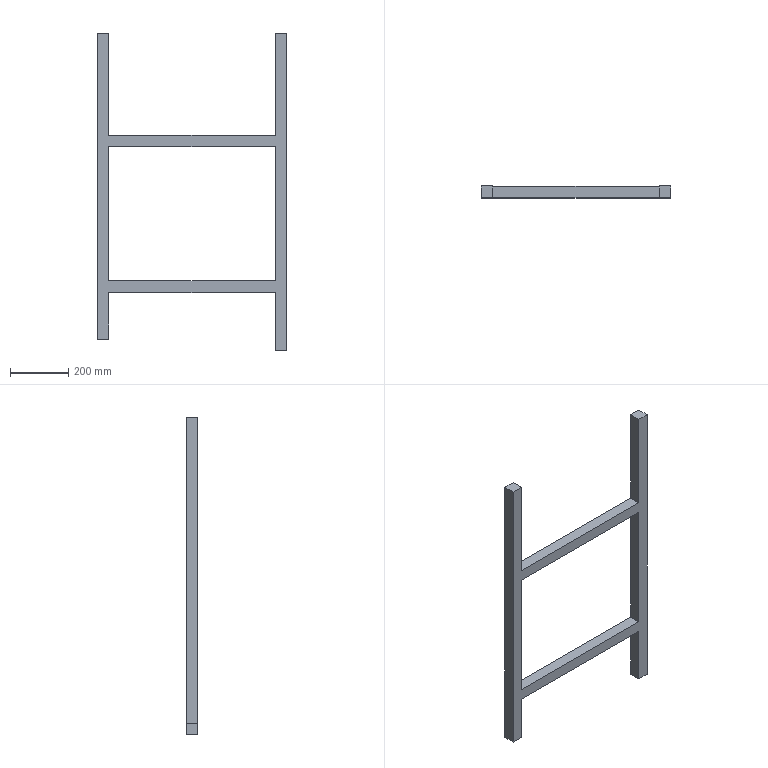Part | NX | features 凸台-拉伸23 2 | 1 solid | 18 faces | box 650 x 40 x 1090 mm | volume 5248000 mm3 | plane 18
STEP:
#1=CARTESIAN_POINT('',(3933.,-40.,-902.985));
#2=VERTEX_POINT('',#1);
#3=CARTESIAN_POINT('',(3933.,0.,-902.985));
#4=VERTEX_POINT('',#3);
#5=CARTESIAN_POINT('',(3933.,0.,-902.985));
#6=DIRECTION('',(0.,1.,0.));
#7=VECTOR('',#6,1000.);
#8=LINE('',#5,#7);
#9=EDGE_CURVE('',#2,#4,#8,.T.);
#10=ORIENTED_EDGE('',*,*,#9,.F.);
#11=CARTESIAN_POINT('',(3363.,-40.,-902.985));
#12=VERTEX_POINT('',#11);
#13=CARTESIAN_POINT('',(3989.569,-40.,-902.985));
#14=DIRECTION('',(-1.,0.,0.));
#15=VECTOR('',#14,1000.);
#16=LINE('',#13,#15);
#17=EDGE_CURVE('',#2,#12,#16,.T.);
#18=ORIENTED_EDGE('',*,*,#17,.T.);
#19=CARTESIAN_POINT('',(3363.,0.,-902.985));
#20=VERTEX_POINT('',#19);
#21=CARTESIAN_POINT('',(3363.,0.,-902.985));
#22=DIRECTION('',(0.,1.,0.));
#23=VECTOR('',#22,1000.);
#24=LINE('',#21,#23);
#25=EDGE_CURVE('',#12,#20,#24,.T.);
#26=ORIENTED_EDGE('',*,*,#25,.T.);
#27=CARTESIAN_POINT('',(3989.569,0.,-902.985));
#28=DIRECTION('',(-1.,0.,0.));
#29=VECTOR('',#28,1000.);
#30=LINE('',#27,#29);
#31=EDGE_CURVE('',#4,#20,#30,.T.);
#32=ORIENTED_EDGE('',*,*,#31,.F.);
#33=EDGE_LOOP('',(#10,#18,#26,#32));
#34=FACE_BOUND('',#33,.T.);
#35=CARTESIAN_POINT('',(3989.569,0.,-902.985));
#36=DIRECTION('',(0.,0.,1.));
#37=DIRECTION('',(1.,0.,0.));
#38=AXIS2_PLACEMENT_3D('',#35,#36,#37);
#39=PLANE('',#38);
#40=ADVANCED_FACE('',(#34),#39,.F.);
#41=CARTESIAN_POINT('',(3933.,0.,-862.985));
#42=VERTEX_POINT('',#41);
#43=CARTESIAN_POINT('',(3933.,-40.,-862.985));
#44=VERTEX_POINT('',#43);
#45=CARTESIAN_POINT('',(3933.,0.,-862.985));
#46=DIRECTION('',(0.,-1.,0.));
#47=VECTOR('',#46,1000.);
#48=LINE('',#45,#47);
#49=EDGE_CURVE('',#42,#44,#48,.T.);
#50=ORIENTED_EDGE('',*,*,#49,.F.);
#51=CARTESIAN_POINT('',(3363.,0.,-862.985));
#52=VERTEX_POINT('',#51);
#53=CARTESIAN_POINT('',(3989.569,0.,-862.985));
#54=DIRECTION('',(-1.,0.,0.));
#55=VECTOR('',#54,1000.);
#56=LINE('',#53,#55);
#57=EDGE_CURVE('',#42,#52,#56,.T.);
#58=ORIENTED_EDGE('',*,*,#57,.T.);
#59=CARTESIAN_POINT('',(3363.,-40.,-862.985));
#60=VERTEX_POINT('',#59);
#61=CARTESIAN_POINT('',(3363.,0.,-862.985));
#62=DIRECTION('',(0.,-1.,0.));
#63=VECTOR('',#62,1000.);
#64=LINE('',#61,#63);
#65=EDGE_CURVE('',#52,#60,#64,.T.);
#66=ORIENTED_EDGE('',*,*,#65,.T.);
#67=CARTESIAN_POINT('',(3989.569,-40.,-862.985));
#68=DIRECTION('',(-1.,0.,0.));
#69=VECTOR('',#68,1000.);
#70=LINE('',#67,#69);
#71=EDGE_CURVE('',#44,#60,#70,.T.);
#72=ORIENTED_EDGE('',*,*,#71,.F.);
#73=EDGE_LOOP('',(#50,#58,#66,#72));
#74=FACE_BOUND('',#73,.T.);
#75=CARTESIAN_POINT('',(3989.569,0.,-862.985));
#76=DIRECTION('',(0.,0.,-1.));
#77=DIRECTION('',(-1.,0.,0.));
#78=AXIS2_PLACEMENT_3D('',#75,#76,#77);
#79=PLANE('',#78);
#80=ADVANCED_FACE('',(#74),#79,.F.);
#81=CARTESIAN_POINT('',(3363.,0.,-12.985));
#82=VERTEX_POINT('',#81);
#83=CARTESIAN_POINT('',(3323.,0.,-12.985));
#84=VERTEX_POINT('',#83);
#85=CARTESIAN_POINT('',(3323.,0.,-12.985));
#86=DIRECTION('',(-1.,0.,0.));
#87=VECTOR('',#86,1000.);
#88=LINE('',#85,#87);
#89=EDGE_CURVE('',#82,#84,#88,.T.);
#90=ORIENTED_EDGE('',*,*,#89,.T.);
#91=CARTESIAN_POINT('',(3323.,-40.,-12.985));
#92=VERTEX_POINT('',#91);
#93=CARTESIAN_POINT('',(3323.,0.,-12.985));
#94=DIRECTION('',(0.,-1.,0.));
#95=VECTOR('',#94,1000.);
#96=LINE('',#93,#95);
#97=EDGE_CURVE('',#84,#92,#96,.T.);
#98=ORIENTED_EDGE('',*,*,#97,.T.);
#99=CARTESIAN_POINT('',(3363.,-40.,-12.985));
#100=VERTEX_POINT('',#99);
#101=CARTESIAN_POINT('',(3323.,-40.,-12.985));
#102=DIRECTION('',(1.,0.,0.));
#103=VECTOR('',#102,1000.);
#104=LINE('',#101,#103);
#105=EDGE_CURVE('',#92,#100,#104,.T.);
#106=ORIENTED_EDGE('',*,*,#105,.T.);
#107=CARTESIAN_POINT('',(3363.,0.,-12.985));
#108=DIRECTION('',(0.,1.,0.));
#109=VECTOR('',#108,1000.);
#110=LINE('',#107,#109);
#111=EDGE_CURVE('',#100,#82,#110,.T.);
#112=ORIENTED_EDGE('',*,*,#111,.T.);
#113=EDGE_LOOP('',(#90,#98,#106,#112));
#114=FACE_BOUND('',#113,.T.);
#115=CARTESIAN_POINT('',(4349.569,0.,-12.985));
#116=DIRECTION('',(0.,0.,1.));
#117=DIRECTION('',(1.,0.,0.));
#118=AXIS2_PLACEMENT_3D('',#115,#116,#117);
#119=PLANE('',#118);
#120=ADVANCED_FACE('',(#114),#119,.T.);
#121=CARTESIAN_POINT('',(3323.,0.,-1062.985));
#122=VERTEX_POINT('',#121);
#123=CARTESIAN_POINT('',(3323.,-40.,-1062.985));
#124=VERTEX_POINT('',#123);
#125=CARTESIAN_POINT('',(3323.,0.,-1062.985));
#126=DIRECTION('',(0.,-1.,0.));
#127=VECTOR('',#126,1000.);
#128=LINE('',#125,#127);
#129=EDGE_CURVE('',#122,#124,#128,.T.);
#130=ORIENTED_EDGE('',*,*,#129,.F.);
#131=CARTESIAN_POINT('',(3363.,0.,-1062.985));
#132=VERTEX_POINT('',#131);
#133=CARTESIAN_POINT('',(3323.,0.,-1062.985));
#134=DIRECTION('',(-1.,0.,0.));
#135=VECTOR('',#134,1000.);
#136=LINE('',#133,#135);
#137=EDGE_CURVE('',#132,#122,#136,.T.);
#138=ORIENTED_EDGE('',*,*,#137,.F.);
#139=CARTESIAN_POINT('',(3363.,-40.,-1062.985));
#140=VERTEX_POINT('',#139);
#141=CARTESIAN_POINT('',(3363.,0.,-1062.985));
#142=DIRECTION('',(0.,1.,0.));
#143=VECTOR('',#142,1000.);
#144=LINE('',#141,#143);
#145=EDGE_CURVE('',#140,#132,#144,.T.);
#146=ORIENTED_EDGE('',*,*,#145,.F.);
#147=CARTESIAN_POINT('',(3323.,-40.,-1062.985));
#148=DIRECTION('',(1.,0.,0.));
#149=VECTOR('',#148,1000.);
#150=LINE('',#147,#149);
#151=EDGE_CURVE('',#124,#140,#150,.T.);
#152=ORIENTED_EDGE('',*,*,#151,.F.);
#153=EDGE_LOOP('',(#130,#138,#146,#152));
#154=FACE_BOUND('',#153,.T.);
#155=CARTESIAN_POINT('',(3000.,0.,-1062.985));
#156=DIRECTION('',(0.,0.,1.));
#157=DIRECTION('',(1.,0.,0.));
#158=AXIS2_PLACEMENT_3D('',#155,#156,#157);
#159=PLANE('',#158);
#160=ADVANCED_FACE('',(#154),#159,.F.);
#161=ORIENTED_EDGE('',*,*,#97,.F.);
#162=CARTESIAN_POINT('',(3323.,0.,43.584));
#163=DIRECTION('',(0.,0.,-1.));
#164=VECTOR('',#163,1000.);
#165=LINE('',#162,#164);
#166=EDGE_CURVE('',#84,#122,#165,.T.);
#167=ORIENTED_EDGE('',*,*,#166,.T.);
#168=ORIENTED_EDGE('',*,*,#129,.T.);
#169=CARTESIAN_POINT('',(3323.,-40.,43.584));
#170=DIRECTION('',(0.,0.,-1.));
#171=VECTOR('',#170,1000.);
#172=LINE('',#169,#171);
#173=EDGE_CURVE('',#92,#124,#172,.T.);
#174=ORIENTED_EDGE('',*,*,#173,.F.);
#175=EDGE_LOOP('',(#161,#167,#168,#174));
#176=FACE_BOUND('',#175,.T.);
#177=CARTESIAN_POINT('',(3323.,0.,43.584));
#178=DIRECTION('',(1.,0.,0.));
#179=DIRECTION('',(0.,1.,0.));
#180=AXIS2_PLACEMENT_3D('',#177,#178,#179);
#181=PLANE('',#180);
#182=ADVANCED_FACE('',(#176),#181,.F.);
#183=CARTESIAN_POINT('',(3363.,0.,-362.985));
#184=VERTEX_POINT('',#183);
#185=CARTESIAN_POINT('',(3363.,-40.,-362.985));
#186=VERTEX_POINT('',#185);
#187=CARTESIAN_POINT('',(3363.,0.,-362.985));
#188=DIRECTION('',(0.,-1.,0.));
#189=VECTOR('',#188,1000.);
#190=LINE('',#187,#189);
#191=EDGE_CURVE('',#184,#186,#190,.T.);
#192=ORIENTED_EDGE('',*,*,#191,.F.);
#193=CARTESIAN_POINT('',(3363.,0.,43.584));
#194=DIRECTION('',(0.,0.,-1.));
#195=VECTOR('',#194,1000.);
#196=LINE('',#193,#195);
#197=EDGE_CURVE('',#82,#184,#196,.T.);
#198=ORIENTED_EDGE('',*,*,#197,.F.);
#199=ORIENTED_EDGE('',*,*,#111,.F.);
#200=CARTESIAN_POINT('',(3363.,-40.,43.584));
#201=DIRECTION('',(0.,0.,-1.));
#202=VECTOR('',#201,1000.);
#203=LINE('',#200,#202);
#204=EDGE_CURVE('',#100,#186,#203,.T.);
#205=ORIENTED_EDGE('',*,*,#204,.T.);
#206=EDGE_LOOP('',(#192,#198,#199,#205));
#207=FACE_BOUND('',#206,.T.);
#208=CARTESIAN_POINT('',(3363.,0.,43.584));
#209=DIRECTION('',(-1.,0.,0.));
#210=DIRECTION('',(0.,-1.,0.));
#211=AXIS2_PLACEMENT_3D('',#208,#209,#210);
#212=PLANE('',#211);
#213=ADVANCED_FACE('',(#207),#212,.F.);
#214=CARTESIAN_POINT('',(3933.,-40.,-402.985));
#215=VERTEX_POINT('',#214);
#216=CARTESIAN_POINT('',(3933.,0.,-402.985));
#217=VERTEX_POINT('',#216);
#218=CARTESIAN_POINT('',(3933.,0.,-402.985));
#219=DIRECTION('',(0.,1.,0.));
#220=VECTOR('',#219,1000.);
#221=LINE('',#218,#220);
#222=EDGE_CURVE('',#215,#217,#221,.T.);
#223=ORIENTED_EDGE('',*,*,#222,.F.);
#224=CARTESIAN_POINT('',(3363.,-40.,-402.985));
#225=VERTEX_POINT('',#224);
#226=CARTESIAN_POINT('',(3989.569,-40.,-402.985));
#227=DIRECTION('',(-1.,0.,0.));
#228=VECTOR('',#227,1000.);
#229=LINE('',#226,#228);
#230=EDGE_CURVE('',#215,#225,#229,.T.);
#231=ORIENTED_EDGE('',*,*,#230,.T.);
#232=CARTESIAN_POINT('',(3363.,0.,-402.985));
#233=VERTEX_POINT('',#232);
#234=CARTESIAN_POINT('',(3363.,0.,-402.985));
#235=DIRECTION('',(0.,1.,0.));
#236=VECTOR('',#235,1000.);
#237=LINE('',#234,#236);
#238=EDGE_CURVE('',#225,#233,#237,.T.);
#239=ORIENTED_EDGE('',*,*,#238,.T.);
#240=CARTESIAN_POINT('',(3989.569,0.,-402.985));
#241=DIRECTION('',(-1.,0.,0.));
#242=VECTOR('',#241,1000.);
#243=LINE('',#240,#242);
#244=EDGE_CURVE('',#217,#233,#243,.T.);
#245=ORIENTED_EDGE('',*,*,#244,.F.);
#246=EDGE_LOOP('',(#223,#231,#239,#245));
#247=FACE_BOUND('',#246,.T.);
#248=CARTESIAN_POINT('',(3989.569,0.,-402.985));
#249=DIRECTION('',(0.,0.,1.));
#250=DIRECTION('',(1.,0.,0.));
#251=AXIS2_PLACEMENT_3D('',#248,#249,#250);
#252=PLANE('',#251);
#253=ADVANCED_FACE('',(#247),#252,.F.);
#254=CARTESIAN_POINT('',(3933.,0.,-362.985));
#255=VERTEX_POINT('',#254);
#256=CARTESIAN_POINT('',(3933.,-40.,-362.985));
#257=VERTEX_POINT('',#256);
#258=CARTESIAN_POINT('',(3933.,0.,-362.985));
#259=DIRECTION('',(0.,-1.,0.));
#260=VECTOR('',#259,1000.);
#261=LINE('',#258,#260);
#262=EDGE_CURVE('',#255,#257,#261,.T.);
#263=ORIENTED_EDGE('',*,*,#262,.F.);
#264=CARTESIAN_POINT('',(3989.569,0.,-362.985));
#265=DIRECTION('',(-1.,0.,0.));
#266=VECTOR('',#265,1000.);
#267=LINE('',#264,#266);
#268=EDGE_CURVE('',#255,#184,#267,.T.);
#269=ORIENTED_EDGE('',*,*,#268,.T.);
#270=ORIENTED_EDGE('',*,*,#191,.T.);
#271=CARTESIAN_POINT('',(3989.569,-40.,-362.985));
#272=DIRECTION('',(-1.,0.,0.));
#273=VECTOR('',#272,1000.);
#274=LINE('',#271,#273);
#275=EDGE_CURVE('',#257,#186,#274,.T.);
#276=ORIENTED_EDGE('',*,*,#275,.F.);
#277=EDGE_LOOP('',(#263,#269,#270,#276));
#278=FACE_BOUND('',#277,.T.);
#279=CARTESIAN_POINT('',(3989.569,0.,-362.985));
#280=DIRECTION('',(0.,0.,-1.));
#281=DIRECTION('',(-1.,0.,0.));
#282=AXIS2_PLACEMENT_3D('',#279,#280,#281);
#283=PLANE('',#282);
#284=ADVANCED_FACE('',(#278),#283,.F.);
#285=CARTESIAN_POINT('',(3973.,0.,-1102.985));
#286=VERTEX_POINT('',#285);
#287=CARTESIAN_POINT('',(3933.,0.,-1102.985));
#288=VERTEX_POINT('',#287);
#289=CARTESIAN_POINT('',(3933.,0.,-1102.985));
#290=DIRECTION('',(-1.,0.,0.));
#291=VECTOR('',#290,1000.);
#292=LINE('',#289,#291);
#293=EDGE_CURVE('',#286,#288,#292,.T.);
#294=ORIENTED_EDGE('',*,*,#293,.F.);
#295=CARTESIAN_POINT('',(3973.,-40.,-1102.985));
#296=VERTEX_POINT('',#295);
#297=CARTESIAN_POINT('',(3973.,-40.,-1102.985));
#298=DIRECTION('',(0.,1.,0.));
#299=VECTOR('',#298,1000.);
#300=LINE('',#297,#299);
#301=EDGE_CURVE('',#296,#286,#300,.T.);
#302=ORIENTED_EDGE('',*,*,#301,.F.);
#303=CARTESIAN_POINT('',(3933.,-40.,-1102.985));
#304=VERTEX_POINT('',#303);
#305=CARTESIAN_POINT('',(3933.,-40.,-1102.985));
#306=DIRECTION('',(1.,0.,0.));
#307=VECTOR('',#306,1000.);
#308=LINE('',#305,#307);
#309=EDGE_CURVE('',#304,#296,#308,.T.);
#310=ORIENTED_EDGE('',*,*,#309,.F.);
#311=CARTESIAN_POINT('',(3933.,-40.,-1102.985));
#312=DIRECTION('',(0.,-1.,0.));
#313=VECTOR('',#312,1000.);
#314=LINE('',#311,#313);
#315=EDGE_CURVE('',#288,#304,#314,.T.);
#316=ORIENTED_EDGE('',*,*,#315,.F.);
#317=EDGE_LOOP('',(#294,#302,#310,#316));
#318=FACE_BOUND('',#317,.T.);
#319=CARTESIAN_POINT('',(4349.569,-560.,-1102.985));
#320=DIRECTION('',(0.,0.,1.));
#321=DIRECTION('',(1.,0.,0.));
#322=AXIS2_PLACEMENT_3D('',#319,#320,#321);
#323=PLANE('',#322);
#324=ADVANCED_FACE('',(#318),#323,.F.);
#325=CARTESIAN_POINT('',(3973.,0.,-12.985));
#326=VERTEX_POINT('',#325);
#327=CARTESIAN_POINT('',(3973.,0.,-1159.553));
#328=DIRECTION('',(0.,0.,1.));
#329=VECTOR('',#328,1000.);
#330=LINE('',#327,#329);
#331=EDGE_CURVE('',#286,#326,#330,.T.);
#332=ORIENTED_EDGE('',*,*,#331,.F.);
#333=ORIENTED_EDGE('',*,*,#293,.T.);
#334=CARTESIAN_POINT('',(3933.,0.,-1159.553));
#335=DIRECTION('',(0.,0.,1.));
#336=VECTOR('',#335,1000.);
#337=LINE('',#334,#336);
#338=EDGE_CURVE('',#288,#4,#337,.T.);
#339=ORIENTED_EDGE('',*,*,#338,.T.);
#340=ORIENTED_EDGE('',*,*,#31,.T.);
#341=CARTESIAN_POINT('',(3363.,0.,43.584));
#342=DIRECTION('',(0.,0.,-1.));
#343=VECTOR('',#342,1000.);
#344=LINE('',#341,#343);
#345=EDGE_CURVE('',#20,#132,#344,.T.);
#346=ORIENTED_EDGE('',*,*,#345,.T.);
#347=ORIENTED_EDGE('',*,*,#137,.T.);
#348=ORIENTED_EDGE('',*,*,#166,.F.);
#349=ORIENTED_EDGE('',*,*,#89,.F.);
#350=ORIENTED_EDGE('',*,*,#197,.T.);
#351=ORIENTED_EDGE('',*,*,#268,.F.);
#352=CARTESIAN_POINT('',(3933.,0.,-12.985));
#353=VERTEX_POINT('',#352);
#354=CARTESIAN_POINT('',(3933.,0.,-1159.553));
#355=DIRECTION('',(0.,0.,1.));
#356=VECTOR('',#355,1000.);
#357=LINE('',#354,#356);
#358=EDGE_CURVE('',#255,#353,#357,.T.);
#359=ORIENTED_EDGE('',*,*,#358,.T.);
#360=CARTESIAN_POINT('',(3933.,0.,-12.985));
#361=DIRECTION('',(1.,0.,0.));
#362=VECTOR('',#361,1000.);
#363=LINE('',#360,#362);
#364=EDGE_CURVE('',#353,#326,#363,.T.);
#365=ORIENTED_EDGE('',*,*,#364,.T.);
#366=EDGE_LOOP('',(#332,#333,#339,#340,#346,#347,#348,#349,#350,#351,#359,#365));
#367=FACE_BOUND('',#366,.T.);
#368=ORIENTED_EDGE('',*,*,#57,.F.);
#369=CARTESIAN_POINT('',(3933.,0.,-1159.553));
#370=DIRECTION('',(0.,0.,1.));
#371=VECTOR('',#370,1000.);
#372=LINE('',#369,#371);
#373=EDGE_CURVE('',#42,#217,#372,.T.);
#374=ORIENTED_EDGE('',*,*,#373,.T.);
#375=ORIENTED_EDGE('',*,*,#244,.T.);
#376=CARTESIAN_POINT('',(3363.,0.,43.584));
#377=DIRECTION('',(0.,0.,-1.));
#378=VECTOR('',#377,1000.);
#379=LINE('',#376,#378);
#380=EDGE_CURVE('',#233,#52,#379,.T.);
#381=ORIENTED_EDGE('',*,*,#380,.T.);
#382=EDGE_LOOP('',(#368,#374,#375,#381));
#383=FACE_BOUND('',#382,.T.);
#384=CARTESIAN_POINT('',(3933.,0.,-1159.553));
#385=DIRECTION('',(0.,-1.,0.));
#386=DIRECTION('',(1.,0.,0.));
#387=AXIS2_PLACEMENT_3D('',#384,#385,#386);
#388=PLANE('',#387);
#389=ADVANCED_FACE('',(#367,#383),#388,.F.);
#390=CARTESIAN_POINT('',(3973.,-40.,-12.985));
#391=VERTEX_POINT('',#390);
#392=CARTESIAN_POINT('',(3973.,-40.,-1159.553));
#393=DIRECTION('',(0.,0.,1.));
#394=VECTOR('',#393,1000.);
#395=LINE('',#392,#394);
#396=EDGE_CURVE('',#296,#391,#395,.T.);
#397=ORIENTED_EDGE('',*,*,#396,.F.);
#398=ORIENTED_EDGE('',*,*,#301,.T.);
#399=ORIENTED_EDGE('',*,*,#331,.T.);
#400=CARTESIAN_POINT('',(3973.,-40.,-12.985));
#401=DIRECTION('',(0.,-1.,0.));
#402=VECTOR('',#401,1000.);
#403=LINE('',#400,#402);
#404=EDGE_CURVE('',#326,#391,#403,.T.);
#405=ORIENTED_EDGE('',*,*,#404,.T.);
#406=EDGE_LOOP('',(#397,#398,#399,#405));
#407=FACE_BOUND('',#406,.T.);
#408=CARTESIAN_POINT('',(3973.,-40.,-1159.553));
#409=DIRECTION('',(-1.,0.,0.));
#410=DIRECTION('',(0.,0.,1.));
#411=AXIS2_PLACEMENT_3D('',#408,#409,#410);
#412=PLANE('',#411);
#413=ADVANCED_FACE('',(#407),#412,.F.);
#414=CARTESIAN_POINT('',(3933.,-40.,-1159.553));
#415=DIRECTION('',(0.,0.,1.));
#416=VECTOR('',#415,1000.);
#417=LINE('',#414,#416);
#418=EDGE_CURVE('',#44,#215,#417,.T.);
#419=ORIENTED_EDGE('',*,*,#418,.F.);
#420=ORIENTED_EDGE('',*,*,#71,.T.);
#421=CARTESIAN_POINT('',(3363.,-40.,43.584));
#422=DIRECTION('',(0.,0.,-1.));
#423=VECTOR('',#422,1000.);
#424=LINE('',#421,#423);
#425=EDGE_CURVE('',#225,#60,#424,.T.);
#426=ORIENTED_EDGE('',*,*,#425,.F.);
#427=ORIENTED_EDGE('',*,*,#230,.F.);
#428=EDGE_LOOP('',(#419,#420,#426,#427));
#429=FACE_BOUND('',#428,.T.);
#430=ORIENTED_EDGE('',*,*,#17,.F.);
#431=CARTESIAN_POINT('',(3933.,-40.,-1159.553));
#432=DIRECTION('',(0.,0.,1.));
#433=VECTOR('',#432,1000.);
#434=LINE('',#431,#433);
#435=EDGE_CURVE('',#304,#2,#434,.T.);
#436=ORIENTED_EDGE('',*,*,#435,.F.);
#437=ORIENTED_EDGE('',*,*,#309,.T.);
#438=ORIENTED_EDGE('',*,*,#396,.T.);
#439=CARTESIAN_POINT('',(3933.,-40.,-12.985));
#440=VERTEX_POINT('',#439);
#441=CARTESIAN_POINT('',(3933.,-40.,-12.985));
#442=DIRECTION('',(-1.,0.,0.));
#443=VECTOR('',#442,1000.);
#444=LINE('',#441,#443);
#445=EDGE_CURVE('',#391,#440,#444,.T.);
#446=ORIENTED_EDGE('',*,*,#445,.T.);
#447=CARTESIAN_POINT('',(3933.,-40.,-1159.553));
#448=DIRECTION('',(0.,0.,1.));
#449=VECTOR('',#448,1000.);
#450=LINE('',#447,#449);
#451=EDGE_CURVE('',#257,#440,#450,.T.);
#452=ORIENTED_EDGE('',*,*,#451,.F.);
#453=ORIENTED_EDGE('',*,*,#275,.T.);
#454=ORIENTED_EDGE('',*,*,#204,.F.);
#455=ORIENTED_EDGE('',*,*,#105,.F.);
#456=ORIENTED_EDGE('',*,*,#173,.T.);
#457=ORIENTED_EDGE('',*,*,#151,.T.);
#458=CARTESIAN_POINT('',(3363.,-40.,43.584));
#459=DIRECTION('',(0.,0.,-1.));
#460=VECTOR('',#459,1000.);
#461=LINE('',#458,#460);
#462=EDGE_CURVE('',#12,#140,#461,.T.);
#463=ORIENTED_EDGE('',*,*,#462,.F.);
#464=EDGE_LOOP('',(#430,#436,#437,#438,#446,#452,#453,#454,#455,#456,#457,#463));
#465=FACE_BOUND('',#464,.T.);
#466=CARTESIAN_POINT('',(3933.,-40.,-1159.553));
#467=DIRECTION('',(0.,1.,0.));
#468=DIRECTION('',(-1.,0.,0.));
#469=AXIS2_PLACEMENT_3D('',#466,#467,#468);
#470=PLANE('',#469);
#471=ADVANCED_FACE('',(#429,#465),#470,.F.);
#472=CARTESIAN_POINT('',(3933.,-40.,-12.985));
#473=DIRECTION('',(0.,1.,0.));
#474=VECTOR('',#473,1000.);
#475=LINE('',#472,#474);
#476=EDGE_CURVE('',#440,#353,#475,.T.);
#477=ORIENTED_EDGE('',*,*,#476,.F.);
#478=ORIENTED_EDGE('',*,*,#445,.F.);
#479=ORIENTED_EDGE('',*,*,#404,.F.);
#480=ORIENTED_EDGE('',*,*,#364,.F.);
#481=EDGE_LOOP('',(#477,#478,#479,#480));
#482=FACE_BOUND('',#481,.T.);
#483=CARTESIAN_POINT('',(3000.,0.,-12.985));
#484=DIRECTION('',(0.,0.,-1.));
#485=DIRECTION('',(-1.,0.,0.));
#486=AXIS2_PLACEMENT_3D('',#483,#484,#485);
#487=PLANE('',#486);
#488=ADVANCED_FACE('',(#482),#487,.F.);
#489=ORIENTED_EDGE('',*,*,#358,.F.);
#490=ORIENTED_EDGE('',*,*,#262,.T.);
#491=ORIENTED_EDGE('',*,*,#451,.T.);
#492=ORIENTED_EDGE('',*,*,#476,.T.);
#493=EDGE_LOOP('',(#489,#490,#491,#492));
#494=FACE_BOUND('',#493,.T.);
#495=CARTESIAN_POINT('',(3933.,-40.,-1159.553));
#496=DIRECTION('',(1.,0.,0.));
#497=DIRECTION('',(0.,0.,-1.));
#498=AXIS2_PLACEMENT_3D('',#495,#496,#497);
#499=PLANE('',#498);
#500=ADVANCED_FACE('',(#494),#499,.F.);
#501=ORIENTED_EDGE('',*,*,#25,.F.);
#502=ORIENTED_EDGE('',*,*,#462,.T.);
#503=ORIENTED_EDGE('',*,*,#145,.T.);
#504=ORIENTED_EDGE('',*,*,#345,.F.);
#505=EDGE_LOOP('',(#501,#502,#503,#504));
#506=FACE_BOUND('',#505,.T.);
#507=CARTESIAN_POINT('',(3363.,0.,43.584));
#508=DIRECTION('',(-1.,0.,0.));
#509=DIRECTION('',(0.,-1.,0.));
#510=AXIS2_PLACEMENT_3D('',#507,#508,#509);
#511=PLANE('',#510);
#512=ADVANCED_FACE('',(#506),#511,.F.);
#513=ORIENTED_EDGE('',*,*,#65,.F.);
#514=ORIENTED_EDGE('',*,*,#380,.F.);
#515=ORIENTED_EDGE('',*,*,#238,.F.);
#516=ORIENTED_EDGE('',*,*,#425,.T.);
#517=EDGE_LOOP('',(#513,#514,#515,#516));
#518=FACE_BOUND('',#517,.T.);
#519=CARTESIAN_POINT('',(3363.,0.,43.584));
#520=DIRECTION('',(-1.,0.,0.));
#521=DIRECTION('',(0.,-1.,0.));
#522=AXIS2_PLACEMENT_3D('',#519,#520,#521);
#523=PLANE('',#522);
#524=ADVANCED_FACE('',(#518),#523,.F.);
#525=ORIENTED_EDGE('',*,*,#9,.T.);
#526=ORIENTED_EDGE('',*,*,#338,.F.);
#527=ORIENTED_EDGE('',*,*,#315,.T.);
#528=ORIENTED_EDGE('',*,*,#435,.T.);
#529=EDGE_LOOP('',(#525,#526,#527,#528));
#530=FACE_BOUND('',#529,.T.);
#531=CARTESIAN_POINT('',(3933.,-40.,-1159.553));
#532=DIRECTION('',(1.,0.,0.));
#533=DIRECTION('',(0.,0.,-1.));
#534=AXIS2_PLACEMENT_3D('',#531,#532,#533);
#535=PLANE('',#534);
#536=ADVANCED_FACE('',(#530),#535,.F.);
#537=ORIENTED_EDGE('',*,*,#49,.T.);
#538=ORIENTED_EDGE('',*,*,#418,.T.);
#539=ORIENTED_EDGE('',*,*,#222,.T.);
#540=ORIENTED_EDGE('',*,*,#373,.F.);
#541=EDGE_LOOP('',(#537,#538,#539,#540));
#542=FACE_BOUND('',#541,.T.);
#543=CARTESIAN_POINT('',(3933.,-40.,-1159.553));
#544=DIRECTION('',(1.,0.,0.));
#545=DIRECTION('',(0.,0.,-1.));
#546=AXIS2_PLACEMENT_3D('',#543,#544,#545);
#547=PLANE('',#546);
#548=ADVANCED_FACE('',(#542),#547,.F.);
#549=CLOSED_SHELL('',(#40,#80,#120,#160,#182,#213,#253,#284,#324,#389,#413,#471,#488,#500,#512,#524,#536,#548));
#550=MANIFOLD_SOLID_BREP('',#549);
#551=(LENGTH_UNIT()NAMED_UNIT(*)SI_UNIT(.MILLI.,.METRE.));
#552=UNCERTAINTY_MEASURE_WITH_UNIT(LENGTH_MEASURE(0.00001),#551,'','');
#553=(NAMED_UNIT(*)PLANE_ANGLE_UNIT()SI_UNIT($,.RADIAN.));
#554=(NAMED_UNIT(*)SI_UNIT($,.STERADIAN.)SOLID_ANGLE_UNIT());
#555=(GEOMETRIC_REPRESENTATION_CONTEXT(3)GLOBAL_UNCERTAINTY_ASSIGNED_CONTEXT((#552))GLOBAL_UNIT_ASSIGNED_CONTEXT((#551,#553,#554))REPRESENTATION_CONTEXT('',''));
#556=ADVANCED_BREP_SHAPE_REPRESENTATION('',(#550),#555);